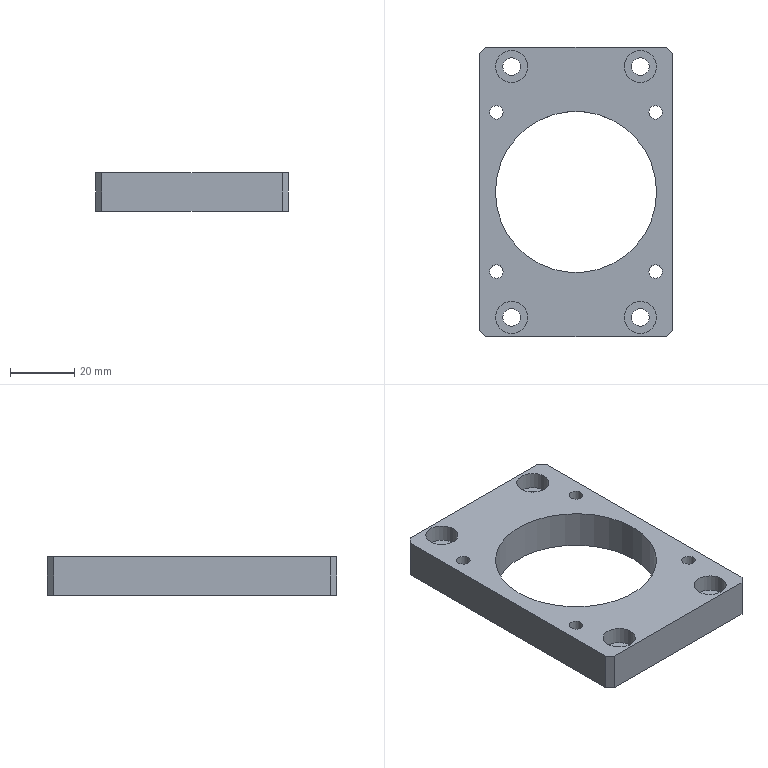CAM job | NX | 3-axis milling, drilling | part box 60 x 90 x 12 mm | stock box 65 x 95 x 15 mm
Tools:
number,name,description,diameter,corner_radius,flute_length,length,flutes
6,D6,平底铣刀-粗,6.0,0.0,25.0,75.0,2
9,D10,平底铣刀-粗,10.0,0.0,35.0,75.0,2
7,D6-J,平底铣刀-精,6.0,0.0,25.0,75.0,2
1,D80R0.8飞刀,圆鼻刀-粗,80.0,0.8,50.0,75.0,2
1,D80R0.8飞刀-J,圆鼻刀-精,80.0,0.8,50.0,75.0,2
2,D6倒角刀,倒角刀,6.0,0.0,3.0,25.0,2
22,M5X0.8,丝锥,4.2,0.0,35.0,50.0,2
17,钻头5.5,Twist Drill 5 mm,5.5,0.0,52.0,54.0,2
14,ZT4.3,Drilling Tool,4.3,0.0,50.0,75.0,4
Operations:
program,operation,operation_type,tool,method,geometry_group,spindle_rpm,surface_speed,feed_per_tooth,feed_cut,feed_plunge,cut_length_mm,path_length_mm,cut_time_min,machine_time_min
B,底壁铣飞面一刀开粗_COPY,VolumeBased25DMillingOperation,D80R0.8飞刀,分层开粗-切深K-步距G,W-B,2800.0,703.696,0.5357,3000.0,100.0,990.97,1956.948,0.3303,0.4269
B,底壁铣飞面一刀精光_COPY,VolumeBased25DMillingOperation,D80R0.8飞刀-J,侧刃精光-切深K-步距G,W-B,4000.0,1005.28,0.125,1000.0,100.0,197.998,293.998,0.198,0.2076
B,C0.3封闭铣廓倒角6X45L_COPY,PlanarMilling,D6倒角刀,爬面_倒角-切深0-步距G,W-B,7000.0,131.0,0.1071,1500.0,100.0,166.229,262.229,0.1108,0.1204
B,钻倒角_1,Operation,D6倒角刀,METHOD,W-B,8000.0,150.796,0.0625,1000.0,0.0,22.8,303.365,0.0228,0.0509
B,铣倒角_3,PlanarMilling,D6倒角刀,METHOD,W-B,8000.0,150.796,0.075,1200.0,100.0,71.178,637.714,0.0593,0.116
B,平面去毛刺6X45L_COPY,SurfaceContour,D6倒角刀,爬面_倒角-切深0-步距G,W-B,6500.0,122.519,0.1154,1500.0,100.0,562.846,1133.496,0.3752,0.4323
A,顶面,FaceMilling,D80R0.8飞刀,侧刃精光-切深K-步距G,W-A,4500.0,1385.0,0.1667,1500.0,100.0,184.0,280.0,0.1227,0.1323
A,外形粗_2,VolumeBased25DMillingOperation,D10,METHOD,W-A,8000.0,251.327,0.375,6000.0,80.0,5566.6,5677.1,0.9278,0.9388
A,底壁铣螺旋开粗-中_COPY,VolumeBased25DMillingOperation,D10,分层开粗-切深K-步距G,W-A,8000.0,251.32,0.25,4000.0,100.0,2652.876,2762.776,0.6632,0.6742
A,打点-深0.8,Operation,D6倒角刀,NONE,W-A,8000.0,150.796,0.0312,500.0,90.0,14.4,325.552,0.0288,0.0599
A,通孔-M5螺纹底孔,Operation,ZT4.3,NONE,W-A,3000.0,40.526,0.025,300.0,90.0,84.0,419.523,0.28,0.3136
A,沉头孔-钻孔0段,Operation,钻头5.5,NONE,W-A,2500.0,43.197,0.06,300.0,90.0,66.609,394.25,0.222,0.2548
A,铣孔开粗D6_1,CylinderMilling,D6,NONE,W-A,8000.0,150.796,0.075,1200.0,100.0,635.598,1213.198,0.5297,0.5874
A,铣孔精光D6_1,CylinderMilling,D6-J,精光步距切深关,W-A,8000.0,150.796,0.0312,500.0,100.0,133.594,713.194,0.2672,0.3251
A,仅选体,SurfaceContour,D6倒角刀,METHOD,W-A,8000.0,150.796,0.1875,3000.0,100.0,471.019,583.788,0.157,0.1683
A,铣倒角_1,PlanarMilling,D6倒角刀,METHOD,W-A,8000.0,150.796,0.0312,500.0,100.0,72.081,624.593,0.1442,0.1994
A,铣倒角_2,PlanarMilling,D6倒角刀,NONE,W-A,8000.0,150.796,0.05,800.0,100.0,161.004,707.569,0.2013,0.2559
A,通孔-攻牙M5,Operation,M5X0.8,METHOD,W-A,500.0,6.597,0.0008,0.8,90.0,66.0,383.523,82.5,82.532
A,外形半精_2,VolumeBased25DMillingOperation,D6-J,METHOD,W-A,9000.0,169.646,0.0667,1200.0,100.0,319.079,442.079,0.2659,0.2782
A,底壁铣精光侧面-中_COPY,VolumeBased25DMillingOperation,D6-J,侧刃精光-切深K-步距G,W-A,8000.0,150.792,0.0625,1000.0,100.0,290.42,332.607,0.2904,0.2946